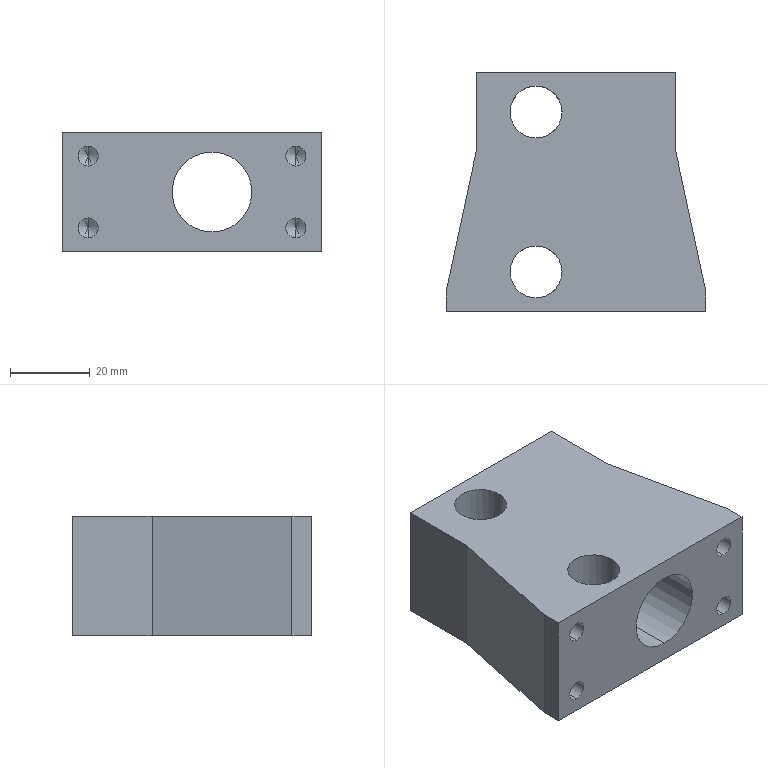Part | STEP file | BU-A11 | 1 solid | 32 faces | box 65 x 60 x 30 mm | volume 72438 mm3 | cylinder 14 | plane 10 | cone 8 | commonest cylinder face diameters 5 x8 13 x4 20 x2